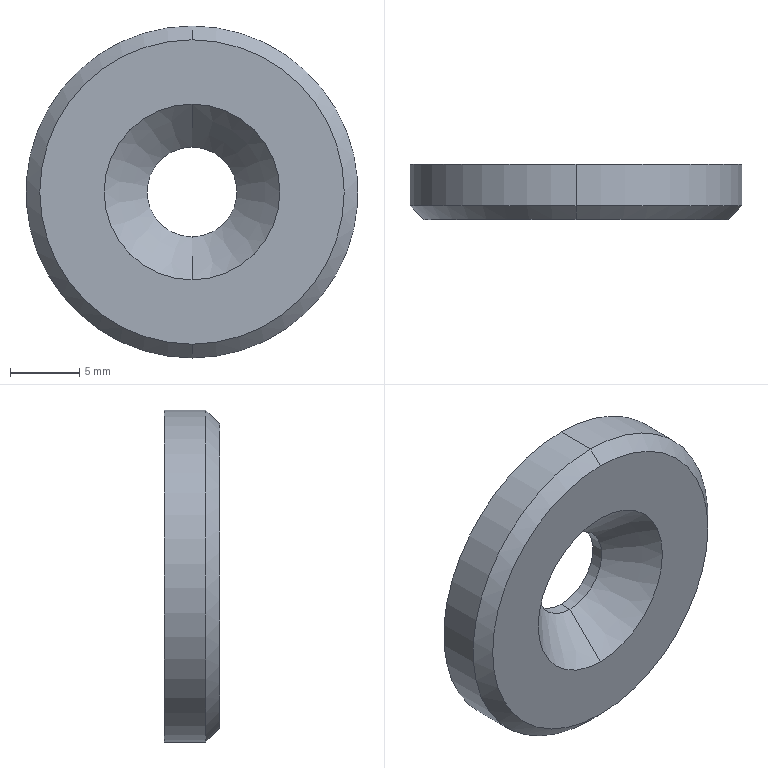Part | STEP file | Standard stop EP - EP - 2A Polimold - M6 | 1 solid | 10 faces | box 24 x 4 x 24 mm | volume 1511 mm3 | cone 4 | cylinder 4 | plane 2 | commonest cylinder face diameters 6.5 x2 24 x2
STEP:
#1=CARTESIAN_POINT('',(0.,0.,0.));
#2=DIRECTION('',(0.,0.,1.));
#3=DIRECTION('',(1.,0.,0.));
#4=AXIS2_PLACEMENT_3D('',#1,#2,#3);
#5=CARTESIAN_POINT('',(0.,0.,-11.));
#6=VERTEX_POINT('',#5);
#7=CARTESIAN_POINT('',(0.,0.,11.));
#8=VERTEX_POINT('',#7);
#9=CARTESIAN_POINT('',(0.,0.,0.));
#10=DIRECTION('',(0.,-1.,0.));
#11=DIRECTION('',(0.,0.,1.));
#12=AXIS2_PLACEMENT_3D('',#9,#10,#11);
#13=CIRCLE('',#12,11.);
#14=CARTESIAN_POINT('',(0.,1.,0.));
#15=DIRECTION('',(0.,1.,0.));
#16=DIRECTION('',(0.,0.,1.));
#17=AXIS2_PLACEMENT_3D('',#14,#15,#16);
#18=CONICAL_SURFACE('',#17,12.,0.7854);
#19=CARTESIAN_POINT('',(6.283,-1.));
#20=DIRECTION('',(-1.,0.));
#21=VECTOR('',#20,1.);
#22=LINE('',#19,#21);
#23=(GEOMETRIC_REPRESENTATION_CONTEXT(2)PARAMETRIC_REPRESENTATION_CONTEXT()REPRESENTATION_CONTEXT('',''));
#24=DEFINITIONAL_REPRESENTATION('',(#22),#23);
#25=PCURVE('',#18,#24);
#26=CARTESIAN_POINT('',(0.,0.,0.));
#27=DIRECTION('',(0.,1.,0.));
#28=DIRECTION('',(0.,0.,1.));
#29=AXIS2_PLACEMENT_3D('',#26,#27,#28);
#30=PLANE('',#29);
#31=CARTESIAN_POINT('',(11.,0.));
#32=CARTESIAN_POINT('',(11.,-19.053));
#33=CARTESIAN_POINT('',(-5.5,-9.526));
#34=CARTESIAN_POINT('',(-22.,0.));
#35=CARTESIAN_POINT('',(-5.5,9.526));
#36=CARTESIAN_POINT('',(11.,19.053));
#37=CARTESIAN_POINT('',(11.,0.));
#38=(BOUNDED_CURVE()B_SPLINE_CURVE(2,(#31,#32,#33,#34,#35,#36,#37),.UNSPECIFIED.,.T.,.F.)B_SPLINE_CURVE_WITH_KNOTS((1,2,2,2,2,1),(-2.094,0.,2.094,4.189,6.283,8.378),.UNSPECIFIED.)CURVE()GEOMETRIC_REPRESENTATION_ITEM()RATIONAL_B_SPLINE_CURVE((1.,0.5,1.,0.5,1.,0.5,1.))REPRESENTATION_ITEM(''));
#39=(GEOMETRIC_REPRESENTATION_CONTEXT(2)PARAMETRIC_REPRESENTATION_CONTEXT()REPRESENTATION_CONTEXT('',''));
#40=DEFINITIONAL_REPRESENTATION('',(#38),#39);
#41=PCURVE('',#30,#40);
#42=SURFACE_CURVE('',#13,(#25,#41),.PCURVE_S1.);
#43=EDGE_CURVE('',#6,#8,#42,.T.);
#44=ORIENTED_EDGE('',*,*,#43,.F.);
#45=CARTESIAN_POINT('',(0.,1.,-12.));
#46=VERTEX_POINT('',#45);
#47=CARTESIAN_POINT('',(0.,1.,-12.));
#48=DIRECTION('',(0.,0.7071,-0.7071));
#49=VECTOR('',#48,1.);
#50=LINE('',#47,#49);
#51=CARTESIAN_POINT('',(3.142,0.));
#52=DIRECTION('',(0.,1.));
#53=VECTOR('',#52,1.);
#54=LINE('',#51,#53);
#55=(GEOMETRIC_REPRESENTATION_CONTEXT(2)PARAMETRIC_REPRESENTATION_CONTEXT()REPRESENTATION_CONTEXT('',''));
#56=DEFINITIONAL_REPRESENTATION('',(#54),#55);
#57=PCURVE('',#18,#56);
#58=CARTESIAN_POINT('',(0.,1.,0.));
#59=DIRECTION('',(0.,1.,0.));
#60=DIRECTION('',(0.,0.,1.));
#61=AXIS2_PLACEMENT_3D('',#58,#59,#60);
#62=CONICAL_SURFACE('',#61,12.,0.7854);
#63=CARTESIAN_POINT('',(3.142,0.));
#64=DIRECTION('',(0.,1.));
#65=VECTOR('',#64,1.);
#66=LINE('',#63,#65);
#67=(GEOMETRIC_REPRESENTATION_CONTEXT(2)PARAMETRIC_REPRESENTATION_CONTEXT()REPRESENTATION_CONTEXT('',''));
#68=DEFINITIONAL_REPRESENTATION('',(#66),#67);
#69=PCURVE('',#62,#68);
#70=SURFACE_CURVE('',#50,(#57,#69),.PCURVE_S1.);
#71=EDGE_CURVE('',#6,#46,#70,.T.);
#72=ORIENTED_EDGE('',*,*,#71,.T.);
#73=CARTESIAN_POINT('',(0.,1.,12.));
#74=VERTEX_POINT('',#73);
#75=CARTESIAN_POINT('',(0.,1.,0.));
#76=DIRECTION('',(0.,1.,0.));
#77=DIRECTION('',(0.,0.,1.));
#78=AXIS2_PLACEMENT_3D('',#75,#76,#77);
#79=CIRCLE('',#78,12.);
#80=CARTESIAN_POINT('',(0.,0.));
#81=DIRECTION('',(1.,0.));
#82=VECTOR('',#81,1.);
#83=LINE('',#80,#82);
#84=(GEOMETRIC_REPRESENTATION_CONTEXT(2)PARAMETRIC_REPRESENTATION_CONTEXT()REPRESENTATION_CONTEXT('',''));
#85=DEFINITIONAL_REPRESENTATION('',(#83),#84);
#86=PCURVE('',#18,#85);
#87=CARTESIAN_POINT('',(0.,4.,0.));
#88=DIRECTION('',(0.,-1.,0.));
#89=DIRECTION('',(0.,0.,-1.));
#90=AXIS2_PLACEMENT_3D('',#87,#88,#89);
#91=CYLINDRICAL_SURFACE('',#90,12.);
#92=CARTESIAN_POINT('',(3.142,3.));
#93=DIRECTION('',(-1.,0.));
#94=VECTOR('',#93,1.);
#95=LINE('',#92,#94);
#96=(GEOMETRIC_REPRESENTATION_CONTEXT(2)PARAMETRIC_REPRESENTATION_CONTEXT()REPRESENTATION_CONTEXT('',''));
#97=DEFINITIONAL_REPRESENTATION('',(#95),#96);
#98=PCURVE('',#91,#97);
#99=SURFACE_CURVE('',#79,(#86,#98),.PCURVE_S1.);
#100=EDGE_CURVE('',#74,#46,#99,.T.);
#101=ORIENTED_EDGE('',*,*,#100,.F.);
#102=CARTESIAN_POINT('',(0.,1.,12.));
#103=DIRECTION('',(0.,0.7071,0.7071));
#104=VECTOR('',#103,1.);
#105=LINE('',#102,#104);
#106=CARTESIAN_POINT('',(0.,0.));
#107=DIRECTION('',(0.,1.));
#108=VECTOR('',#107,1.);
#109=LINE('',#106,#108);
#110=(GEOMETRIC_REPRESENTATION_CONTEXT(2)PARAMETRIC_REPRESENTATION_CONTEXT()REPRESENTATION_CONTEXT('',''));
#111=DEFINITIONAL_REPRESENTATION('',(#109),#110);
#112=PCURVE('',#18,#111);
#113=CARTESIAN_POINT('',(6.283,0.));
#114=DIRECTION('',(0.,1.));
#115=VECTOR('',#114,1.);
#116=LINE('',#113,#115);
#117=(GEOMETRIC_REPRESENTATION_CONTEXT(2)PARAMETRIC_REPRESENTATION_CONTEXT()REPRESENTATION_CONTEXT('',''));
#118=DEFINITIONAL_REPRESENTATION('',(#116),#117);
#119=PCURVE('',#62,#118);
#120=SURFACE_CURVE('',#105,(#112,#119),.PCURVE_S1.);
#121=EDGE_CURVE('',#8,#74,#120,.T.);
#122=ORIENTED_EDGE('',*,*,#121,.F.);
#123=EDGE_LOOP('',(#44,#72,#101,#122));
#124=FACE_BOUND('',#123,.T.);
#125=ADVANCED_FACE('',(#124),#18,.T.);
#126=CARTESIAN_POINT('',(0.,3.1,-3.25));
#127=VERTEX_POINT('',#126);
#128=CARTESIAN_POINT('',(0.,0.,-6.35));
#129=VERTEX_POINT('',#128);
#130=CARTESIAN_POINT('',(0.,0.,-6.35));
#131=DIRECTION('',(0.,-0.7071,-0.7071));
#132=VECTOR('',#131,1.);
#133=LINE('',#130,#132);
#134=CARTESIAN_POINT('',(0.,0.,0.));
#135=DIRECTION('',(0.,-1.,0.));
#136=DIRECTION('',(0.,0.,-1.));
#137=AXIS2_PLACEMENT_3D('',#134,#135,#136);
#138=CONICAL_SURFACE('',#137,6.35,0.7854);
#139=CARTESIAN_POINT('',(6.283,0.));
#140=DIRECTION('',(0.,1.));
#141=VECTOR('',#140,1.);
#142=LINE('',#139,#141);
#143=(GEOMETRIC_REPRESENTATION_CONTEXT(2)PARAMETRIC_REPRESENTATION_CONTEXT()REPRESENTATION_CONTEXT('',''));
#144=DEFINITIONAL_REPRESENTATION('',(#142),#143);
#145=PCURVE('',#138,#144);
#146=CARTESIAN_POINT('',(0.,0.,0.));
#147=DIRECTION('',(0.,-1.,0.));
#148=DIRECTION('',(0.,0.,-1.));
#149=AXIS2_PLACEMENT_3D('',#146,#147,#148);
#150=CONICAL_SURFACE('',#149,6.35,0.7854);
#151=CARTESIAN_POINT('',(0.,0.));
#152=DIRECTION('',(0.,1.));
#153=VECTOR('',#152,1.);
#154=LINE('',#151,#153);
#155=(GEOMETRIC_REPRESENTATION_CONTEXT(2)PARAMETRIC_REPRESENTATION_CONTEXT()REPRESENTATION_CONTEXT('',''));
#156=DEFINITIONAL_REPRESENTATION('',(#154),#155);
#157=PCURVE('',#150,#156);
#158=SURFACE_CURVE('',#133,(#145,#157),.PCURVE_S1.);
#159=EDGE_CURVE('',#127,#129,#158,.T.);
#160=ORIENTED_EDGE('',*,*,#159,.T.);
#161=CARTESIAN_POINT('',(0.,0.,6.35));
#162=VERTEX_POINT('',#161);
#163=CARTESIAN_POINT('',(0.,0.,0.));
#164=DIRECTION('',(0.,-1.,0.));
#165=DIRECTION('',(0.,0.,-1.));
#166=AXIS2_PLACEMENT_3D('',#163,#164,#165);
#167=CIRCLE('',#166,6.35);
#168=CARTESIAN_POINT('',(0.,0.));
#169=DIRECTION('',(1.,0.));
#170=VECTOR('',#169,1.);
#171=LINE('',#168,#170);
#172=(GEOMETRIC_REPRESENTATION_CONTEXT(2)PARAMETRIC_REPRESENTATION_CONTEXT()REPRESENTATION_CONTEXT('',''));
#173=DEFINITIONAL_REPRESENTATION('',(#171),#172);
#174=PCURVE('',#138,#173);
#175=CARTESIAN_POINT('',(-6.35,0.));
#176=CARTESIAN_POINT('',(-6.35,10.999));
#177=CARTESIAN_POINT('',(3.175,5.499));
#178=CARTESIAN_POINT('',(12.7,0.));
#179=CARTESIAN_POINT('',(3.175,-5.499));
#180=CARTESIAN_POINT('',(-6.35,-10.999));
#181=CARTESIAN_POINT('',(-6.35,0.));
#182=(BOUNDED_CURVE()B_SPLINE_CURVE(2,(#175,#176,#177,#178,#179,#180,#181),.UNSPECIFIED.,.T.,.F.)B_SPLINE_CURVE_WITH_KNOTS((1,2,2,2,2,1),(-2.094,0.,2.094,4.189,6.283,8.378),.UNSPECIFIED.)CURVE()GEOMETRIC_REPRESENTATION_ITEM()RATIONAL_B_SPLINE_CURVE((1.,0.5,1.,0.5,1.,0.5,1.))REPRESENTATION_ITEM(''));
#183=(GEOMETRIC_REPRESENTATION_CONTEXT(2)PARAMETRIC_REPRESENTATION_CONTEXT()REPRESENTATION_CONTEXT('',''));
#184=DEFINITIONAL_REPRESENTATION('',(#182),#183);
#185=PCURVE('',#30,#184);
#186=SURFACE_CURVE('',#167,(#174,#185),.PCURVE_S1.);
#187=EDGE_CURVE('',#162,#129,#186,.T.);
#188=ORIENTED_EDGE('',*,*,#187,.F.);
#189=CARTESIAN_POINT('',(0.,3.1,3.25));
#190=VERTEX_POINT('',#189);
#191=CARTESIAN_POINT('',(0.,0.,6.35));
#192=DIRECTION('',(0.,-0.7071,0.7071));
#193=VECTOR('',#192,1.);
#194=LINE('',#191,#193);
#195=CARTESIAN_POINT('',(3.142,0.));
#196=DIRECTION('',(0.,1.));
#197=VECTOR('',#196,1.);
#198=LINE('',#195,#197);
#199=(GEOMETRIC_REPRESENTATION_CONTEXT(2)PARAMETRIC_REPRESENTATION_CONTEXT()REPRESENTATION_CONTEXT('',''));
#200=DEFINITIONAL_REPRESENTATION('',(#198),#199);
#201=PCURVE('',#138,#200);
#202=CARTESIAN_POINT('',(3.142,0.));
#203=DIRECTION('',(0.,1.));
#204=VECTOR('',#203,1.);
#205=LINE('',#202,#204);
#206=(GEOMETRIC_REPRESENTATION_CONTEXT(2)PARAMETRIC_REPRESENTATION_CONTEXT()REPRESENTATION_CONTEXT('',''));
#207=DEFINITIONAL_REPRESENTATION('',(#205),#206);
#208=PCURVE('',#150,#207);
#209=SURFACE_CURVE('',#194,(#201,#208),.PCURVE_S1.);
#210=EDGE_CURVE('',#190,#162,#209,.T.);
#211=ORIENTED_EDGE('',*,*,#210,.F.);
#212=CARTESIAN_POINT('',(0.,3.1,0.));
#213=DIRECTION('',(0.,-1.,0.));
#214=DIRECTION('',(0.,0.,-1.));
#215=AXIS2_PLACEMENT_3D('',#212,#213,#214);
#216=CIRCLE('',#215,3.25);
#217=CARTESIAN_POINT('',(0.,-3.1));
#218=DIRECTION('',(1.,0.));
#219=VECTOR('',#218,1.);
#220=LINE('',#217,#219);
#221=(GEOMETRIC_REPRESENTATION_CONTEXT(2)PARAMETRIC_REPRESENTATION_CONTEXT()REPRESENTATION_CONTEXT('',''));
#222=DEFINITIONAL_REPRESENTATION('',(#220),#221);
#223=PCURVE('',#138,#222);
#224=CARTESIAN_POINT('',(0.,0.,0.));
#225=DIRECTION('',(0.,-1.,0.));
#226=DIRECTION('',(0.,0.,-1.));
#227=AXIS2_PLACEMENT_3D('',#224,#225,#226);
#228=CYLINDRICAL_SURFACE('',#227,3.25);
#229=CARTESIAN_POINT('',(0.,-3.1));
#230=DIRECTION('',(1.,0.));
#231=VECTOR('',#230,1.);
#232=LINE('',#229,#231);
#233=(GEOMETRIC_REPRESENTATION_CONTEXT(2)PARAMETRIC_REPRESENTATION_CONTEXT()REPRESENTATION_CONTEXT('',''));
#234=DEFINITIONAL_REPRESENTATION('',(#232),#233);
#235=PCURVE('',#228,#234);
#236=SURFACE_CURVE('',#216,(#223,#235),.PCURVE_S1.);
#237=EDGE_CURVE('',#190,#127,#236,.T.);
#238=ORIENTED_EDGE('',*,*,#237,.T.);
#239=EDGE_LOOP('',(#160,#188,#211,#238));
#240=FACE_BOUND('',#239,.F.);
#241=ADVANCED_FACE('',(#240),#138,.F.);
#242=CARTESIAN_POINT('',(0.,4.,-3.25));
#243=VERTEX_POINT('',#242);
#244=CARTESIAN_POINT('',(0.,0.,-3.25));
#245=DIRECTION('',(0.,-1.,0.));
#246=VECTOR('',#245,1.);
#247=LINE('',#244,#246);
#248=CARTESIAN_POINT('',(6.283,0.));
#249=DIRECTION('',(0.,1.));
#250=VECTOR('',#249,1.);
#251=LINE('',#248,#250);
#252=(GEOMETRIC_REPRESENTATION_CONTEXT(2)PARAMETRIC_REPRESENTATION_CONTEXT()REPRESENTATION_CONTEXT('',''));
#253=DEFINITIONAL_REPRESENTATION('',(#251),#252);
#254=PCURVE('',#228,#253);
#255=CARTESIAN_POINT('',(0.,0.,0.));
#256=DIRECTION('',(0.,-1.,0.));
#257=DIRECTION('',(0.,0.,-1.));
#258=AXIS2_PLACEMENT_3D('',#255,#256,#257);
#259=CYLINDRICAL_SURFACE('',#258,3.25);
#260=CARTESIAN_POINT('',(0.,0.));
#261=DIRECTION('',(0.,1.));
#262=VECTOR('',#261,1.);
#263=LINE('',#260,#262);
#264=(GEOMETRIC_REPRESENTATION_CONTEXT(2)PARAMETRIC_REPRESENTATION_CONTEXT()REPRESENTATION_CONTEXT('',''));
#265=DEFINITIONAL_REPRESENTATION('',(#263),#264);
#266=PCURVE('',#259,#265);
#267=SURFACE_CURVE('',#247,(#254,#266),.PCURVE_S1.);
#268=EDGE_CURVE('',#243,#127,#267,.T.);
#269=ORIENTED_EDGE('',*,*,#268,.T.);
#270=ORIENTED_EDGE('',*,*,#237,.F.);
#271=CARTESIAN_POINT('',(0.,4.,3.25));
#272=VERTEX_POINT('',#271);
#273=CARTESIAN_POINT('',(0.,0.,3.25));
#274=DIRECTION('',(0.,-1.,0.));
#275=VECTOR('',#274,1.);
#276=LINE('',#273,#275);
#277=CARTESIAN_POINT('',(3.142,0.));
#278=DIRECTION('',(0.,1.));
#279=VECTOR('',#278,1.);
#280=LINE('',#277,#279);
#281=(GEOMETRIC_REPRESENTATION_CONTEXT(2)PARAMETRIC_REPRESENTATION_CONTEXT()REPRESENTATION_CONTEXT('',''));
#282=DEFINITIONAL_REPRESENTATION('',(#280),#281);
#283=PCURVE('',#228,#282);
#284=CARTESIAN_POINT('',(3.142,0.));
#285=DIRECTION('',(0.,1.));
#286=VECTOR('',#285,1.);
#287=LINE('',#284,#286);
#288=(GEOMETRIC_REPRESENTATION_CONTEXT(2)PARAMETRIC_REPRESENTATION_CONTEXT()REPRESENTATION_CONTEXT('',''));
#289=DEFINITIONAL_REPRESENTATION('',(#287),#288);
#290=PCURVE('',#259,#289);
#291=SURFACE_CURVE('',#276,(#283,#290),.PCURVE_S1.);
#292=EDGE_CURVE('',#272,#190,#291,.T.);
#293=ORIENTED_EDGE('',*,*,#292,.F.);
#294=CARTESIAN_POINT('',(0.,4.,0.));
#295=DIRECTION('',(0.,-1.,0.));
#296=DIRECTION('',(0.,0.,-1.));
#297=AXIS2_PLACEMENT_3D('',#294,#295,#296);
#298=CIRCLE('',#297,3.25);
#299=CARTESIAN_POINT('',(0.,-4.));
#300=DIRECTION('',(1.,0.));
#301=VECTOR('',#300,1.);
#302=LINE('',#299,#301);
#303=(GEOMETRIC_REPRESENTATION_CONTEXT(2)PARAMETRIC_REPRESENTATION_CONTEXT()REPRESENTATION_CONTEXT('',''));
#304=DEFINITIONAL_REPRESENTATION('',(#302),#303);
#305=PCURVE('',#228,#304);
#306=CARTESIAN_POINT('',(0.,4.,0.));
#307=DIRECTION('',(0.,1.,0.));
#308=DIRECTION('',(0.,0.,1.));
#309=AXIS2_PLACEMENT_3D('',#306,#307,#308);
#310=PLANE('',#309);
#311=CARTESIAN_POINT('',(-3.25,0.));
#312=CARTESIAN_POINT('',(-3.25,5.629));
#313=CARTESIAN_POINT('',(1.625,2.815));
#314=CARTESIAN_POINT('',(6.5,0.));
#315=CARTESIAN_POINT('',(1.625,-2.815));
#316=CARTESIAN_POINT('',(-3.25,-5.629));
#317=CARTESIAN_POINT('',(-3.25,0.));
#318=(BOUNDED_CURVE()B_SPLINE_CURVE(2,(#311,#312,#313,#314,#315,#316,#317),.UNSPECIFIED.,.T.,.F.)B_SPLINE_CURVE_WITH_KNOTS((1,2,2,2,2,1),(-2.094,0.,2.094,4.189,6.283,8.378),.UNSPECIFIED.)CURVE()GEOMETRIC_REPRESENTATION_ITEM()RATIONAL_B_SPLINE_CURVE((1.,0.5,1.,0.5,1.,0.5,1.))REPRESENTATION_ITEM(''));
#319=(GEOMETRIC_REPRESENTATION_CONTEXT(2)PARAMETRIC_REPRESENTATION_CONTEXT()REPRESENTATION_CONTEXT('',''));
#320=DEFINITIONAL_REPRESENTATION('',(#318),#319);
#321=PCURVE('',#310,#320);
#322=SURFACE_CURVE('',#298,(#305,#321),.PCURVE_S1.);
#323=EDGE_CURVE('',#272,#243,#322,.T.);
#324=ORIENTED_EDGE('',*,*,#323,.T.);
#325=EDGE_LOOP('',(#269,#270,#293,#324));
#326=FACE_BOUND('',#325,.F.);
#327=ADVANCED_FACE('',(#326),#228,.F.);
#328=CARTESIAN_POINT('',(0.,4.,12.));
#329=VERTEX_POINT('',#328);
#330=CARTESIAN_POINT('',(0.,4.,-12.));
#331=VERTEX_POINT('',#330);
#332=CARTESIAN_POINT('',(0.,4.,0.));
#333=DIRECTION('',(0.,1.,0.));
#334=DIRECTION('',(0.,0.,1.));
#335=AXIS2_PLACEMENT_3D('',#332,#333,#334);
#336=CIRCLE('',#335,12.);
#337=CARTESIAN_POINT('',(3.142,0.));
#338=DIRECTION('',(-1.,0.));
#339=VECTOR('',#338,1.);
#340=LINE('',#337,#339);
#341=(GEOMETRIC_REPRESENTATION_CONTEXT(2)PARAMETRIC_REPRESENTATION_CONTEXT()REPRESENTATION_CONTEXT('',''));
#342=DEFINITIONAL_REPRESENTATION('',(#340),#341);
#343=PCURVE('',#91,#342);
#344=CARTESIAN_POINT('',(0.,0.));
#345=DIRECTION('',(1.,0.));
#346=AXIS2_PLACEMENT_2D('',#344,#345);
#347=CIRCLE('',#346,12.);
#348=(GEOMETRIC_REPRESENTATION_CONTEXT(2)PARAMETRIC_REPRESENTATION_CONTEXT()REPRESENTATION_CONTEXT('',''));
#349=DEFINITIONAL_REPRESENTATION('',(#347),#348);
#350=PCURVE('',#310,#349);
#351=SURFACE_CURVE('',#336,(#343,#350),.PCURVE_S1.);
#352=EDGE_CURVE('',#329,#331,#351,.T.);
#353=ORIENTED_EDGE('',*,*,#352,.F.);
#354=CARTESIAN_POINT('',(0.,4.,12.));
#355=DIRECTION('',(0.,-1.,0.));
#356=VECTOR('',#355,1.);
#357=LINE('',#354,#356);
#358=CARTESIAN_POINT('',(3.142,0.));
#359=DIRECTION('',(0.,1.));
#360=VECTOR('',#359,1.);
#361=LINE('',#358,#360);
#362=(GEOMETRIC_REPRESENTATION_CONTEXT(2)PARAMETRIC_REPRESENTATION_CONTEXT()REPRESENTATION_CONTEXT('',''));
#363=DEFINITIONAL_REPRESENTATION('',(#361),#362);
#364=PCURVE('',#91,#363);
#365=CARTESIAN_POINT('',(0.,4.,0.));
#366=DIRECTION('',(0.,-1.,0.));
#367=DIRECTION('',(0.,0.,-1.));
#368=AXIS2_PLACEMENT_3D('',#365,#366,#367);
#369=CYLINDRICAL_SURFACE('',#368,12.);
#370=CARTESIAN_POINT('',(3.142,0.));
#371=DIRECTION('',(0.,1.));
#372=VECTOR('',#371,1.);
#373=LINE('',#370,#372);
#374=(GEOMETRIC_REPRESENTATION_CONTEXT(2)PARAMETRIC_REPRESENTATION_CONTEXT()REPRESENTATION_CONTEXT('',''));
#375=DEFINITIONAL_REPRESENTATION('',(#373),#374);
#376=PCURVE('',#369,#375);
#377=SURFACE_CURVE('',#357,(#364,#376),.PCURVE_S1.);
#378=EDGE_CURVE('',#329,#74,#377,.T.);
#379=ORIENTED_EDGE('',*,*,#378,.T.);
#380=ORIENTED_EDGE('',*,*,#100,.T.);
#381=CARTESIAN_POINT('',(0.,4.,-12.));
#382=DIRECTION('',(0.,-1.,0.));
#383=VECTOR('',#382,1.);
#384=LINE('',#381,#383);
#385=CARTESIAN_POINT('',(0.,0.));
#386=DIRECTION('',(0.,1.));
#387=VECTOR('',#386,1.);
#388=LINE('',#385,#387);
#389=(GEOMETRIC_REPRESENTATION_CONTEXT(2)PARAMETRIC_REPRESENTATION_CONTEXT()REPRESENTATION_CONTEXT('',''));
#390=DEFINITIONAL_REPRESENTATION('',(#388),#389);
#391=PCURVE('',#91,#390);
#392=CARTESIAN_POINT('',(6.283,0.));
#393=DIRECTION('',(0.,1.));
#394=VECTOR('',#393,1.);
#395=LINE('',#392,#394);
#396=(GEOMETRIC_REPRESENTATION_CONTEXT(2)PARAMETRIC_REPRESENTATION_CONTEXT()REPRESENTATION_CONTEXT('',''));
#397=DEFINITIONAL_REPRESENTATION('',(#395),#396);
#398=PCURVE('',#369,#397);
#399=SURFACE_CURVE('',#384,(#391,#398),.PCURVE_S1.);
#400=EDGE_CURVE('',#331,#46,#399,.T.);
#401=ORIENTED_EDGE('',*,*,#400,.F.);
#402=EDGE_LOOP('',(#353,#379,#380,#401));
#403=FACE_BOUND('',#402,.T.);
#404=ADVANCED_FACE('',(#403),#91,.T.);
#405=ORIENTED_EDGE('',*,*,#378,.F.);
#406=CARTESIAN_POINT('',(0.,4.,0.));
#407=DIRECTION('',(0.,1.,0.));
#408=DIRECTION('',(0.,0.,1.));
#409=AXIS2_PLACEMENT_3D('',#406,#407,#408);
#410=CIRCLE('',#409,12.);
#411=CARTESIAN_POINT('',(9.425,0.));
#412=DIRECTION('',(-1.,0.));
#413=VECTOR('',#412,1.);
#414=LINE('',#411,#413);
#415=(GEOMETRIC_REPRESENTATION_CONTEXT(2)PARAMETRIC_REPRESENTATION_CONTEXT()REPRESENTATION_CONTEXT('',''));
#416=DEFINITIONAL_REPRESENTATION('',(#414),#415);
#417=PCURVE('',#369,#416);
#418=CARTESIAN_POINT('',(0.,0.));
#419=DIRECTION('',(1.,0.));
#420=AXIS2_PLACEMENT_2D('',#418,#419);
#421=CIRCLE('',#420,12.);
#422=(GEOMETRIC_REPRESENTATION_CONTEXT(2)PARAMETRIC_REPRESENTATION_CONTEXT()REPRESENTATION_CONTEXT('',''));
#423=DEFINITIONAL_REPRESENTATION('',(#421),#422);
#424=PCURVE('',#310,#423);
#425=SURFACE_CURVE('',#410,(#417,#424),.PCURVE_S1.);
#426=EDGE_CURVE('',#331,#329,#425,.T.);
#427=ORIENTED_EDGE('',*,*,#426,.F.);
#428=ORIENTED_EDGE('',*,*,#400,.T.);
#429=CARTESIAN_POINT('',(0.,1.,0.));
#430=DIRECTION('',(0.,1.,0.));
#431=DIRECTION('',(0.,0.,1.));
#432=AXIS2_PLACEMENT_3D('',#429,#430,#431);
#433=CIRCLE('',#432,12.);
#434=CARTESIAN_POINT('',(9.425,3.));
#435=DIRECTION('',(-1.,0.));
#436=VECTOR('',#435,1.);
#437=LINE('',#434,#436);
#438=(GEOMETRIC_REPRESENTATION_CONTEXT(2)PARAMETRIC_REPRESENTATION_CONTEXT()REPRESENTATION_CONTEXT('',''));
#439=DEFINITIONAL_REPRESENTATION('',(#437),#438);
#440=PCURVE('',#369,#439);
#441=CARTESIAN_POINT('',(0.,0.));
#442=DIRECTION('',(1.,0.));
#443=VECTOR('',#442,1.);
#444=LINE('',#441,#443);
#445=(GEOMETRIC_REPRESENTATION_CONTEXT(2)PARAMETRIC_REPRESENTATION_CONTEXT()REPRESENTATION_CONTEXT('',''));
#446=DEFINITIONAL_REPRESENTATION('',(#444),#445);
#447=PCURVE('',#62,#446);
#448=SURFACE_CURVE('',#433,(#440,#447),.PCURVE_S1.);
#449=EDGE_CURVE('',#46,#74,#448,.T.);
#450=ORIENTED_EDGE('',*,*,#449,.T.);
#451=EDGE_LOOP('',(#405,#427,#428,#450));
#452=FACE_BOUND('',#451,.T.);
#453=ADVANCED_FACE('',(#452),#369,.T.);
#454=CARTESIAN_POINT('',(0.,4.,0.));
#455=DIRECTION('',(0.,-1.,0.));
#456=DIRECTION('',(0.,0.,-1.));
#457=AXIS2_PLACEMENT_3D('',#454,#455,#456);
#458=CIRCLE('',#457,3.25);
#459=CARTESIAN_POINT('',(-3.25,0.));
#460=CARTESIAN_POINT('',(-3.25,5.629));
#461=CARTESIAN_POINT('',(1.625,2.815));
#462=CARTESIAN_POINT('',(6.5,0.));
#463=CARTESIAN_POINT('',(1.625,-2.815));
#464=CARTESIAN_POINT('',(-3.25,-5.629));
#465=CARTESIAN_POINT('',(-3.25,0.));
#466=(BOUNDED_CURVE()B_SPLINE_CURVE(2,(#459,#460,#461,#462,#463,#464,#465),.UNSPECIFIED.,.T.,.F.)B_SPLINE_CURVE_WITH_KNOTS((1,2,2,2,2,1),(-2.094,0.,2.094,4.189,6.283,8.378),.UNSPECIFIED.)CURVE()GEOMETRIC_REPRESENTATION_ITEM()RATIONAL_B_SPLINE_CURVE((1.,0.5,1.,0.5,1.,0.5,1.))REPRESENTATION_ITEM(''));
#467=(GEOMETRIC_REPRESENTATION_CONTEXT(2)PARAMETRIC_REPRESENTATION_CONTEXT()REPRESENTATION_CONTEXT('',''));
#468=DEFINITIONAL_REPRESENTATION('',(#466),#467);
#469=PCURVE('',#310,#468);
#470=CARTESIAN_POINT('',(0.,-4.));
#471=DIRECTION('',(1.,0.));
#472=VECTOR('',#471,1.);
#473=LINE('',#470,#472);
#474=(GEOMETRIC_REPRESENTATION_CONTEXT(2)PARAMETRIC_REPRESENTATION_CONTEXT()REPRESENTATION_CONTEXT('',''));
#475=DEFINITIONAL_REPRESENTATION('',(#473),#474);
#476=PCURVE('',#259,#475);
#477=SURFACE_CURVE('',#458,(#469,#476),.PCURVE_S1.);
#478=EDGE_CURVE('',#243,#272,#477,.T.);
#479=ORIENTED_EDGE('',*,*,#478,.T.);
#480=ORIENTED_EDGE('',*,*,#323,.T.);
#481=EDGE_LOOP('',(#479,#480));
#482=FACE_BOUND('',#481,.T.);
#483=ORIENTED_EDGE('',*,*,#426,.T.);
#484=ORIENTED_EDGE('',*,*,#352,.T.);
#485=EDGE_LOOP('',(#483,#484));
#486=FACE_BOUND('',#485,.T.);
#487=ADVANCED_FACE('',(#482,#486),#310,.T.);
#488=CARTESIAN_POINT('',(0.,0.,0.));
#489=DIRECTION('',(0.,-1.,0.));
#490=DIRECTION('',(0.,0.,1.));
#491=AXIS2_PLACEMENT_3D('',#488,#489,#490);
#492=CIRCLE('',#491,11.);
#493=CARTESIAN_POINT('',(11.,0.));
#494=CARTESIAN_POINT('',(11.,-19.053));
#495=CARTESIAN_POINT('',(-5.5,-9.526));
#496=CARTESIAN_POINT('',(-22.,0.));
#497=CARTESIAN_POINT('',(-5.5,9.526));
#498=CARTESIAN_POINT('',(11.,19.053));
#499=CARTESIAN_POINT('',(11.,0.));
#500=(BOUNDED_CURVE()B_SPLINE_CURVE(2,(#493,#494,#495,#496,#497,#498,#499),.UNSPECIFIED.,.T.,.F.)B_SPLINE_CURVE_WITH_KNOTS((1,2,2,2,2,1),(-2.094,0.,2.094,4.189,6.283,8.378),.UNSPECIFIED.)CURVE()GEOMETRIC_REPRESENTATION_ITEM()RATIONAL_B_SPLINE_CURVE((1.,0.5,1.,0.5,1.,0.5,1.))REPRESENTATION_ITEM(''));
#501=(GEOMETRIC_REPRESENTATION_CONTEXT(2)PARAMETRIC_REPRESENTATION_CONTEXT()REPRESENTATION_CONTEXT('',''));
#502=DEFINITIONAL_REPRESENTATION('',(#500),#501);
#503=PCURVE('',#30,#502);
#504=CARTESIAN_POINT('',(6.283,-1.));
#505=DIRECTION('',(-1.,0.));
#506=VECTOR('',#505,1.);
#507=LINE('',#504,#506);
#508=(GEOMETRIC_REPRESENTATION_CONTEXT(2)PARAMETRIC_REPRESENTATION_CONTEXT()REPRESENTATION_CONTEXT('',''));
#509=DEFINITIONAL_REPRESENTATION('',(#507),#508);
#510=PCURVE('',#62,#509);
#511=SURFACE_CURVE('',#492,(#503,#510),.PCURVE_S1.);
#512=EDGE_CURVE('',#8,#6,#511,.T.);
#513=ORIENTED_EDGE('',*,*,#512,.T.);
#514=ORIENTED_EDGE('',*,*,#43,.T.);
#515=EDGE_LOOP('',(#513,#514));
#516=FACE_BOUND('',#515,.T.);
#517=CARTESIAN_POINT('',(0.,0.,0.));
#518=DIRECTION('',(0.,-1.,0.));
#519=DIRECTION('',(0.,0.,-1.));
#520=AXIS2_PLACEMENT_3D('',#517,#518,#519);
#521=CIRCLE('',#520,6.35);
#522=CARTESIAN_POINT('',(-6.35,0.));
#523=CARTESIAN_POINT('',(-6.35,10.999));
#524=CARTESIAN_POINT('',(3.175,5.499));
#525=CARTESIAN_POINT('',(12.7,0.));
#526=CARTESIAN_POINT('',(3.175,-5.499));
#527=CARTESIAN_POINT('',(-6.35,-10.999));
#528=CARTESIAN_POINT('',(-6.35,0.));
#529=(BOUNDED_CURVE()B_SPLINE_CURVE(2,(#522,#523,#524,#525,#526,#527,#528),.UNSPECIFIED.,.T.,.F.)B_SPLINE_CURVE_WITH_KNOTS((1,2,2,2,2,1),(-2.094,0.,2.094,4.189,6.283,8.378),.UNSPECIFIED.)CURVE()GEOMETRIC_REPRESENTATION_ITEM()RATIONAL_B_SPLINE_CURVE((1.,0.5,1.,0.5,1.,0.5,1.))REPRESENTATION_ITEM(''));
#530=(GEOMETRIC_REPRESENTATION_CONTEXT(2)PARAMETRIC_REPRESENTATION_CONTEXT()REPRESENTATION_CONTEXT('',''));
#531=DEFINITIONAL_REPRESENTATION('',(#529),#530);
#532=PCURVE('',#30,#531);
#533=CARTESIAN_POINT('',(0.,0.));
#534=DIRECTION('',(1.,0.));
#535=VECTOR('',#534,1.);
#536=LINE('',#533,#535);
#537=(GEOMETRIC_REPRESENTATION_CONTEXT(2)PARAMETRIC_REPRESENTATION_CONTEXT()REPRESENTATION_CONTEXT('',''));
#538=DEFINITIONAL_REPRESENTATION('',(#536),#537);
#539=PCURVE('',#150,#538);
#540=SURFACE_CURVE('',#521,(#532,#539),.PCURVE_S1.);
#541=EDGE_CURVE('',#129,#162,#540,.T.);
#542=ORIENTED_EDGE('',*,*,#541,.F.);
#543=ORIENTED_EDGE('',*,*,#187,.F.);
#544=EDGE_LOOP('',(#542,#543));
#545=FACE_BOUND('',#544,.T.);
#546=ADVANCED_FACE('',(#516,#545),#30,.F.);
#547=CARTESIAN_POINT('',(0.,3.1,0.));
#548=DIRECTION('',(0.,-1.,0.));
#549=DIRECTION('',(0.,0.,-1.));
#550=AXIS2_PLACEMENT_3D('',#547,#548,#549);
#551=CIRCLE('',#550,3.25);
#552=CARTESIAN_POINT('',(0.,-3.1));
#553=DIRECTION('',(1.,0.));
#554=VECTOR('',#553,1.);
#555=LINE('',#552,#554);
#556=(GEOMETRIC_REPRESENTATION_CONTEXT(2)PARAMETRIC_REPRESENTATION_CONTEXT()REPRESENTATION_CONTEXT('',''));
#557=DEFINITIONAL_REPRESENTATION('',(#555),#556);
#558=PCURVE('',#259,#557);
#559=CARTESIAN_POINT('',(0.,-3.1));
#560=DIRECTION('',(1.,0.));
#561=VECTOR('',#560,1.);
#562=LINE('',#559,#561);
#563=(GEOMETRIC_REPRESENTATION_CONTEXT(2)PARAMETRIC_REPRESENTATION_CONTEXT()REPRESENTATION_CONTEXT('',''));
#564=DEFINITIONAL_REPRESENTATION('',(#562),#563);
#565=PCURVE('',#150,#564);
#566=SURFACE_CURVE('',#551,(#558,#565),.PCURVE_S1.);
#567=EDGE_CURVE('',#127,#190,#566,.T.);
#568=ORIENTED_EDGE('',*,*,#567,.F.);
#569=ORIENTED_EDGE('',*,*,#268,.F.);
#570=ORIENTED_EDGE('',*,*,#478,.T.);
#571=ORIENTED_EDGE('',*,*,#292,.T.);
#572=EDGE_LOOP('',(#568,#569,#570,#571));
#573=FACE_BOUND('',#572,.F.);
#574=ADVANCED_FACE('',(#573),#259,.F.);
#575=ORIENTED_EDGE('',*,*,#541,.F.);
#576=ORIENTED_EDGE('',*,*,#159,.F.);
#577=ORIENTED_EDGE('',*,*,#567,.T.);
#578=ORIENTED_EDGE('',*,*,#210,.T.);
#579=EDGE_LOOP('',(#575,#576,#577,#578));
#580=FACE_BOUND('',#579,.F.);
#581=ADVANCED_FACE('',(#580),#150,.F.);
#582=ORIENTED_EDGE('',*,*,#71,.F.);
#583=ORIENTED_EDGE('',*,*,#512,.F.);
#584=ORIENTED_EDGE('',*,*,#121,.T.);
#585=ORIENTED_EDGE('',*,*,#449,.F.);
#586=EDGE_LOOP('',(#582,#583,#584,#585));
#587=FACE_BOUND('',#586,.T.);
#588=ADVANCED_FACE('',(#587),#62,.T.);
#589=CLOSED_SHELL('',(#125,#241,#327,#404,#453,#487,#546,#574,#581,#588));
#590=MANIFOLD_SOLID_BREP('',#589);
#591=(LENGTH_UNIT()NAMED_UNIT(*)SI_UNIT(.MILLI.,.METRE.));
#592=UNCERTAINTY_MEASURE_WITH_UNIT(LENGTH_MEASURE(0.0000001),#591,'','');
#593=(NAMED_UNIT(*)PLANE_ANGLE_UNIT()SI_UNIT($,.RADIAN.));
#594=(NAMED_UNIT(*)SI_UNIT($,.STERADIAN.)SOLID_ANGLE_UNIT());
#595=(GEOMETRIC_REPRESENTATION_CONTEXT(3)GLOBAL_UNCERTAINTY_ASSIGNED_CONTEXT((#592))GLOBAL_UNIT_ASSIGNED_CONTEXT((#591,#593,#594))REPRESENTATION_CONTEXT('',''));
#596=ADVANCED_BREP_SHAPE_REPRESENTATION('',(#4,#590),#595);